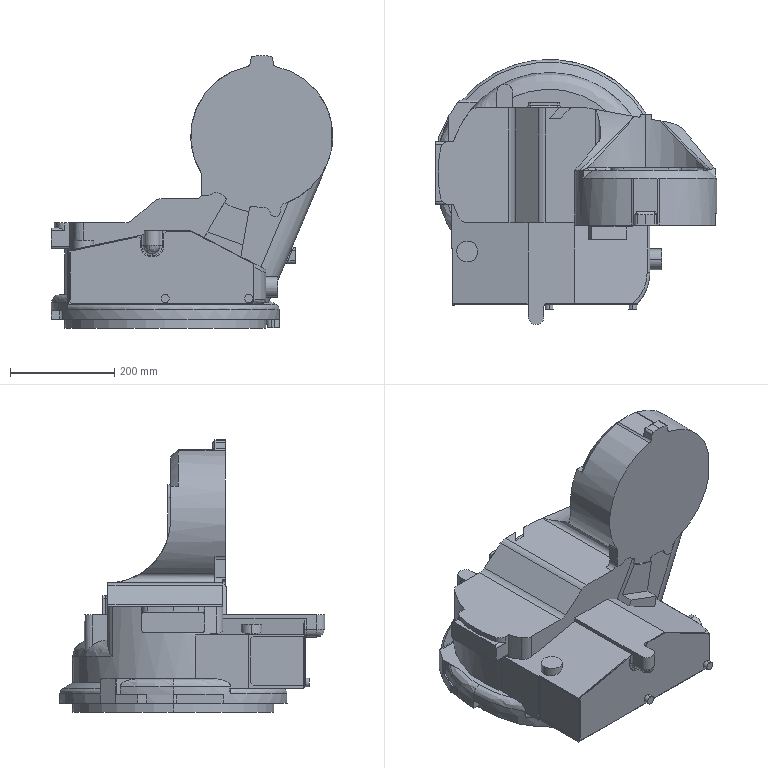Part | STEP file | Link1 | 1 solid | 264 faces | box 539 x 508 x 522 mm | volume 37862681 mm3 | plane 128 | cylinder 103 | spline 21 | cone 7 | torus 5 | commonest cylinder face diameters 10 x25 20 x12 30 x11 6 x10 40 x8 16 x4